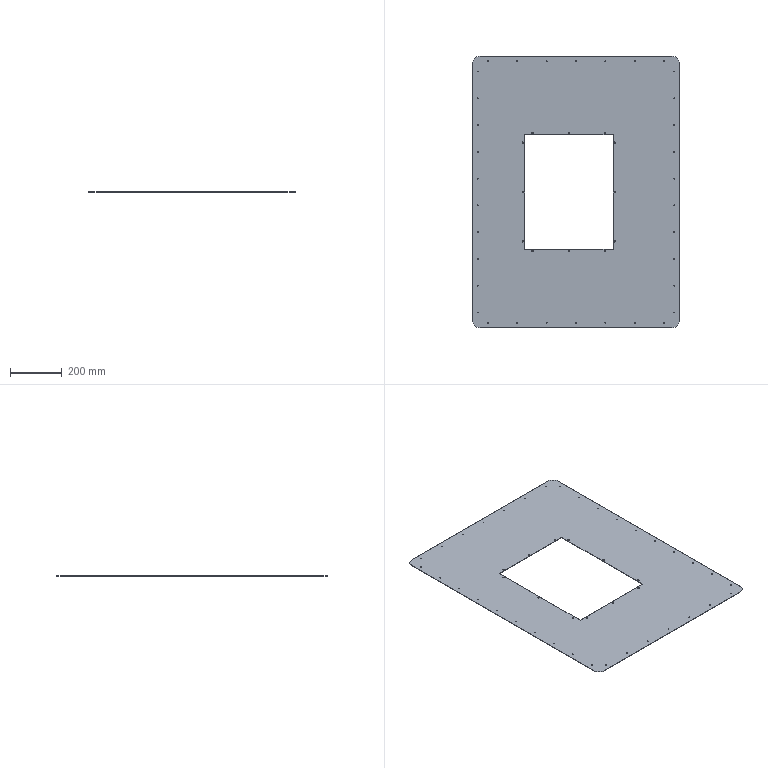Part | STEP file | HESS-408-70-15W-W-42-upper door closing plate 1 | 1 solid | 106 faces | box 796 x 1046 x 1.5 mm | volume 1022602 mm3 | cylinder 96 | plane 10 | commonest cylinder face diameters 3.2 x68 5 x24 60 x4